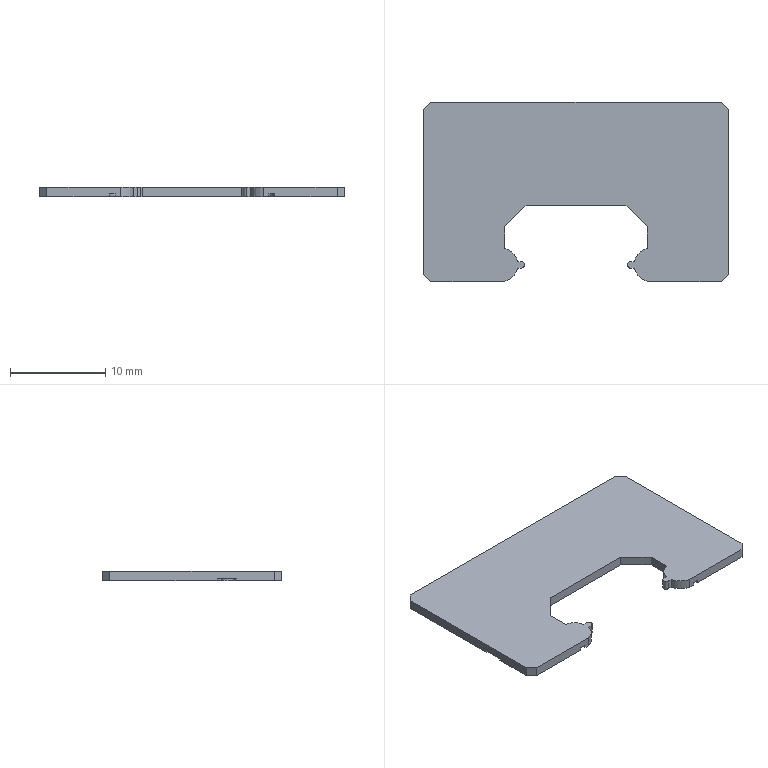Part | STEP file | 10 | 1 solid | 96 faces | box 32 x 18.8 x 1 mm | volume 485.961 mm3 | plane 68 | cylinder 28 | commonest cylinder face diameters 1.3 x4 1.9 x4 3.1 x4 3.5 x4 0.7 x3 1.1 x3